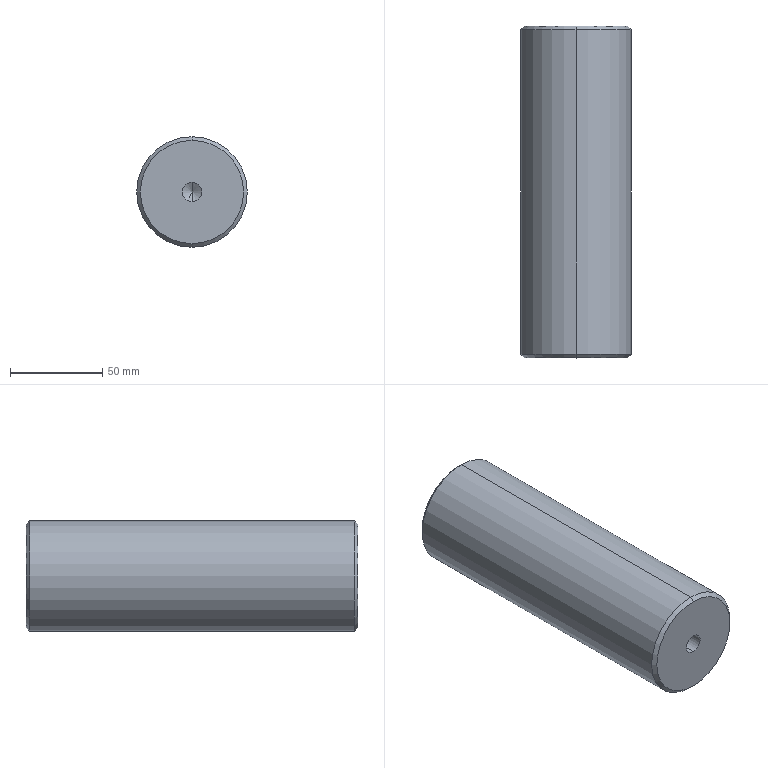Part | STEP file | Pilar - Torre - 1 cav. | 1 solid | 12 faces | box 60 x 180 x 60 mm | volume 505945 mm3 | cone 6 | cylinder 4 | plane 2 | commonest cylinder face diameters 10.5 x2 60 x2
STEP:
#1=CARTESIAN_POINT('',(0.,0.,0.));
#2=DIRECTION('',(0.,0.,1.));
#3=DIRECTION('',(1.,0.,0.));
#4=AXIS2_PLACEMENT_3D('',#1,#2,#3);
#5=CARTESIAN_POINT('',(0.,25.,-5.25));
#6=VERTEX_POINT('',#5);
#7=CARTESIAN_POINT('',(0.,0.,-5.25));
#8=VERTEX_POINT('',#7);
#9=CARTESIAN_POINT('',(0.,0.,-5.25));
#10=DIRECTION('',(0.,-1.,0.));
#11=VECTOR('',#10,1.);
#12=LINE('',#9,#11);
#13=CARTESIAN_POINT('',(0.,0.,0.));
#14=DIRECTION('',(0.,-1.,0.));
#15=DIRECTION('',(0.,0.,-1.));
#16=AXIS2_PLACEMENT_3D('',#13,#14,#15);
#17=CYLINDRICAL_SURFACE('',#16,5.25);
#18=CARTESIAN_POINT('',(6.283,0.));
#19=DIRECTION('',(0.,1.));
#20=VECTOR('',#19,1.);
#21=LINE('',#18,#20);
#22=(GEOMETRIC_REPRESENTATION_CONTEXT(2)PARAMETRIC_REPRESENTATION_CONTEXT()REPRESENTATION_CONTEXT('',''));
#23=DEFINITIONAL_REPRESENTATION('',(#21),#22);
#24=PCURVE('',#17,#23);
#25=CARTESIAN_POINT('',(0.,0.,0.));
#26=DIRECTION('',(0.,-1.,0.));
#27=DIRECTION('',(0.,0.,-1.));
#28=AXIS2_PLACEMENT_3D('',#25,#26,#27);
#29=CYLINDRICAL_SURFACE('',#28,5.25);
#30=CARTESIAN_POINT('',(0.,0.));
#31=DIRECTION('',(0.,1.));
#32=VECTOR('',#31,1.);
#33=LINE('',#30,#32);
#34=(GEOMETRIC_REPRESENTATION_CONTEXT(2)PARAMETRIC_REPRESENTATION_CONTEXT()REPRESENTATION_CONTEXT('',''));
#35=DEFINITIONAL_REPRESENTATION('',(#33),#34);
#36=PCURVE('',#29,#35);
#37=SURFACE_CURVE('',#12,(#24,#36),.PCURVE_S1.);
#38=EDGE_CURVE('',#6,#8,#37,.T.);
#39=ORIENTED_EDGE('',*,*,#38,.T.);
#40=CARTESIAN_POINT('',(0.,0.,5.25));
#41=VERTEX_POINT('',#40);
#42=CARTESIAN_POINT('',(0.,0.,0.));
#43=DIRECTION('',(0.,-1.,0.));
#44=DIRECTION('',(0.,0.,-1.));
#45=AXIS2_PLACEMENT_3D('',#42,#43,#44);
#46=CIRCLE('',#45,5.25);
#47=CARTESIAN_POINT('',(0.,0.));
#48=DIRECTION('',(1.,0.));
#49=VECTOR('',#48,1.);
#50=LINE('',#47,#49);
#51=(GEOMETRIC_REPRESENTATION_CONTEXT(2)PARAMETRIC_REPRESENTATION_CONTEXT()REPRESENTATION_CONTEXT('',''));
#52=DEFINITIONAL_REPRESENTATION('',(#50),#51);
#53=PCURVE('',#17,#52);
#54=CARTESIAN_POINT('',(0.,0.,0.));
#55=DIRECTION('',(0.,1.,0.));
#56=DIRECTION('',(0.,0.,1.));
#57=AXIS2_PLACEMENT_3D('',#54,#55,#56);
#58=PLANE('',#57);
#59=CARTESIAN_POINT('',(-5.25,0.));
#60=CARTESIAN_POINT('',(-5.25,9.093));
#61=CARTESIAN_POINT('',(2.625,4.547));
#62=CARTESIAN_POINT('',(10.5,0.));
#63=CARTESIAN_POINT('',(2.625,-4.547));
#64=CARTESIAN_POINT('',(-5.25,-9.093));
#65=CARTESIAN_POINT('',(-5.25,0.));
#66=(BOUNDED_CURVE()B_SPLINE_CURVE(2,(#59,#60,#61,#62,#63,#64,#65),.UNSPECIFIED.,.T.,.F.)B_SPLINE_CURVE_WITH_KNOTS((1,2,2,2,2,1),(-2.094,0.,2.094,4.189,6.283,8.378),.UNSPECIFIED.)CURVE()GEOMETRIC_REPRESENTATION_ITEM()RATIONAL_B_SPLINE_CURVE((1.,0.5,1.,0.5,1.,0.5,1.))REPRESENTATION_ITEM(''));
#67=(GEOMETRIC_REPRESENTATION_CONTEXT(2)PARAMETRIC_REPRESENTATION_CONTEXT()REPRESENTATION_CONTEXT('',''));
#68=DEFINITIONAL_REPRESENTATION('',(#66),#67);
#69=PCURVE('',#58,#68);
#70=SURFACE_CURVE('',#46,(#53,#69),.PCURVE_S1.);
#71=EDGE_CURVE('',#41,#8,#70,.T.);
#72=ORIENTED_EDGE('',*,*,#71,.F.);
#73=CARTESIAN_POINT('',(0.,25.,5.25));
#74=VERTEX_POINT('',#73);
#75=CARTESIAN_POINT('',(0.,0.,5.25));
#76=DIRECTION('',(0.,-1.,0.));
#77=VECTOR('',#76,1.);
#78=LINE('',#75,#77);
#79=CARTESIAN_POINT('',(3.142,0.));
#80=DIRECTION('',(0.,1.));
#81=VECTOR('',#80,1.);
#82=LINE('',#79,#81);
#83=(GEOMETRIC_REPRESENTATION_CONTEXT(2)PARAMETRIC_REPRESENTATION_CONTEXT()REPRESENTATION_CONTEXT('',''));
#84=DEFINITIONAL_REPRESENTATION('',(#82),#83);
#85=PCURVE('',#17,#84);
#86=CARTESIAN_POINT('',(3.142,0.));
#87=DIRECTION('',(0.,1.));
#88=VECTOR('',#87,1.);
#89=LINE('',#86,#88);
#90=(GEOMETRIC_REPRESENTATION_CONTEXT(2)PARAMETRIC_REPRESENTATION_CONTEXT()REPRESENTATION_CONTEXT('',''));
#91=DEFINITIONAL_REPRESENTATION('',(#89),#90);
#92=PCURVE('',#29,#91);
#93=SURFACE_CURVE('',#78,(#85,#92),.PCURVE_S1.);
#94=EDGE_CURVE('',#74,#41,#93,.T.);
#95=ORIENTED_EDGE('',*,*,#94,.F.);
#96=CARTESIAN_POINT('',(0.,25.,0.));
#97=DIRECTION('',(0.,-1.,0.));
#98=DIRECTION('',(0.,0.,-1.));
#99=AXIS2_PLACEMENT_3D('',#96,#97,#98);
#100=CIRCLE('',#99,5.25);
#101=CARTESIAN_POINT('',(0.,-25.));
#102=DIRECTION('',(1.,0.));
#103=VECTOR('',#102,1.);
#104=LINE('',#101,#103);
#105=(GEOMETRIC_REPRESENTATION_CONTEXT(2)PARAMETRIC_REPRESENTATION_CONTEXT()REPRESENTATION_CONTEXT('',''));
#106=DEFINITIONAL_REPRESENTATION('',(#104),#105);
#107=PCURVE('',#17,#106);
#108=CARTESIAN_POINT('',(0.,25.,0.));
#109=DIRECTION('',(0.,-1.,0.));
#110=DIRECTION('',(0.,0.,-1.));
#111=AXIS2_PLACEMENT_3D('',#108,#109,#110);
#112=CONICAL_SURFACE('',#111,5.25,1.03);
#113=CARTESIAN_POINT('',(0.,0.));
#114=DIRECTION('',(1.,0.));
#115=VECTOR('',#114,1.);
#116=LINE('',#113,#115);
#117=(GEOMETRIC_REPRESENTATION_CONTEXT(2)PARAMETRIC_REPRESENTATION_CONTEXT()REPRESENTATION_CONTEXT('',''));
#118=DEFINITIONAL_REPRESENTATION('',(#116),#117);
#119=PCURVE('',#112,#118);
#120=SURFACE_CURVE('',#100,(#107,#119),.PCURVE_S1.);
#121=EDGE_CURVE('',#74,#6,#120,.T.);
#122=ORIENTED_EDGE('',*,*,#121,.T.);
#123=EDGE_LOOP('',(#39,#72,#95,#122));
#124=FACE_BOUND('',#123,.F.);
#125=ADVANCED_FACE('',(#124),#17,.F.);
#126=ORIENTED_EDGE('',*,*,#121,.F.);
#127=CARTESIAN_POINT('',(0.,28.155,0.));
#128=VERTEX_POINT('',#127);
#129=CARTESIAN_POINT('',(0.,25.,5.25));
#130=DIRECTION('',(0.,-0.515,0.8572));
#131=VECTOR('',#130,1.);
#132=LINE('',#129,#131);
#133=CARTESIAN_POINT('',(3.142,0.));
#134=DIRECTION('',(0.,1.));
#135=VECTOR('',#134,1.);
#136=LINE('',#133,#135);
#137=(GEOMETRIC_REPRESENTATION_CONTEXT(2)PARAMETRIC_REPRESENTATION_CONTEXT()REPRESENTATION_CONTEXT('',''));
#138=DEFINITIONAL_REPRESENTATION('',(#136),#137);
#139=PCURVE('',#112,#138);
#140=CARTESIAN_POINT('',(0.,25.,0.));
#141=DIRECTION('',(0.,-1.,0.));
#142=DIRECTION('',(0.,0.,-1.));
#143=AXIS2_PLACEMENT_3D('',#140,#141,#142);
#144=CONICAL_SURFACE('',#143,5.25,1.03);
#145=CARTESIAN_POINT('',(3.142,0.));
#146=DIRECTION('',(0.,1.));
#147=VECTOR('',#146,1.);
#148=LINE('',#145,#147);
#149=(GEOMETRIC_REPRESENTATION_CONTEXT(2)PARAMETRIC_REPRESENTATION_CONTEXT()REPRESENTATION_CONTEXT('',''));
#150=DEFINITIONAL_REPRESENTATION('',(#148),#149);
#151=PCURVE('',#144,#150);
#152=SURFACE_CURVE('',#132,(#139,#151),.PCURVE_S1.);
#153=EDGE_CURVE('',#128,#74,#152,.T.);
#154=ORIENTED_EDGE('',*,*,#153,.F.);
#155=CARTESIAN_POINT('',(0.,25.,-5.25));
#156=DIRECTION('',(0.,-0.515,-0.8572));
#157=VECTOR('',#156,1.);
#158=LINE('',#155,#157);
#159=CARTESIAN_POINT('',(6.283,0.));
#160=DIRECTION('',(0.,1.));
#161=VECTOR('',#160,1.);
#162=LINE('',#159,#161);
#163=(GEOMETRIC_REPRESENTATION_CONTEXT(2)PARAMETRIC_REPRESENTATION_CONTEXT()REPRESENTATION_CONTEXT('',''));
#164=DEFINITIONAL_REPRESENTATION('',(#162),#163);
#165=PCURVE('',#112,#164);
#166=CARTESIAN_POINT('',(0.,0.));
#167=DIRECTION('',(0.,1.));
#168=VECTOR('',#167,1.);
#169=LINE('',#166,#168);
#170=(GEOMETRIC_REPRESENTATION_CONTEXT(2)PARAMETRIC_REPRESENTATION_CONTEXT()REPRESENTATION_CONTEXT('',''));
#171=DEFINITIONAL_REPRESENTATION('',(#169),#170);
#172=PCURVE('',#144,#171);
#173=SURFACE_CURVE('',#158,(#165,#172),.PCURVE_S1.);
#174=EDGE_CURVE('',#128,#6,#173,.T.);
#175=ORIENTED_EDGE('',*,*,#174,.T.);
#176=EDGE_LOOP('',(#126,#154,#175));
#177=FACE_BOUND('',#176,.F.);
#178=ADVANCED_FACE('',(#177),#112,.F.);
#179=CARTESIAN_POINT('',(0.,180.,28.));
#180=VERTEX_POINT('',#179);
#181=CARTESIAN_POINT('',(0.,180.,-28.));
#182=VERTEX_POINT('',#181);
#183=CARTESIAN_POINT('',(0.,180.,0.));
#184=DIRECTION('',(0.,1.,0.));
#185=DIRECTION('',(0.,0.,1.));
#186=AXIS2_PLACEMENT_3D('',#183,#184,#185);
#187=CIRCLE('',#186,28.);
#188=CARTESIAN_POINT('',(0.,180.,0.));
#189=DIRECTION('',(0.,-1.,0.));
#190=DIRECTION('',(0.,0.,-1.));
#191=AXIS2_PLACEMENT_3D('',#188,#189,#190);
#192=CONICAL_SURFACE('',#191,28.,0.7854);
#193=CARTESIAN_POINT('',(3.142,0.));
#194=DIRECTION('',(-1.,0.));
#195=VECTOR('',#194,1.);
#196=LINE('',#193,#195);
#197=(GEOMETRIC_REPRESENTATION_CONTEXT(2)PARAMETRIC_REPRESENTATION_CONTEXT()REPRESENTATION_CONTEXT('',''));
#198=DEFINITIONAL_REPRESENTATION('',(#196),#197);
#199=PCURVE('',#192,#198);
#200=CARTESIAN_POINT('',(0.,180.,0.));
#201=DIRECTION('',(0.,1.,0.));
#202=DIRECTION('',(0.,0.,1.));
#203=AXIS2_PLACEMENT_3D('',#200,#201,#202);
#204=PLANE('',#203);
#205=CARTESIAN_POINT('',(0.,0.));
#206=DIRECTION('',(1.,0.));
#207=AXIS2_PLACEMENT_2D('',#205,#206);
#208=CIRCLE('',#207,28.);
#209=(GEOMETRIC_REPRESENTATION_CONTEXT(2)PARAMETRIC_REPRESENTATION_CONTEXT()REPRESENTATION_CONTEXT('',''));
#210=DEFINITIONAL_REPRESENTATION('',(#208),#209);
#211=PCURVE('',#204,#210);
#212=SURFACE_CURVE('',#187,(#199,#211),.PCURVE_S1.);
#213=EDGE_CURVE('',#180,#182,#212,.T.);
#214=ORIENTED_EDGE('',*,*,#213,.F.);
#215=CARTESIAN_POINT('',(0.,178.,30.));
#216=VERTEX_POINT('',#215);
#217=CARTESIAN_POINT('',(0.,180.,28.));
#218=DIRECTION('',(0.,-0.7071,0.7071));
#219=VECTOR('',#218,1.);
#220=LINE('',#217,#219);
#221=CARTESIAN_POINT('',(3.142,0.));
#222=DIRECTION('',(0.,1.));
#223=VECTOR('',#222,1.);
#224=LINE('',#221,#223);
#225=(GEOMETRIC_REPRESENTATION_CONTEXT(2)PARAMETRIC_REPRESENTATION_CONTEXT()REPRESENTATION_CONTEXT('',''));
#226=DEFINITIONAL_REPRESENTATION('',(#224),#225);
#227=PCURVE('',#192,#226);
#228=CARTESIAN_POINT('',(0.,180.,0.));
#229=DIRECTION('',(0.,-1.,0.));
#230=DIRECTION('',(0.,0.,-1.));
#231=AXIS2_PLACEMENT_3D('',#228,#229,#230);
#232=CONICAL_SURFACE('',#231,28.,0.7854);
#233=CARTESIAN_POINT('',(3.142,0.));
#234=DIRECTION('',(0.,1.));
#235=VECTOR('',#234,1.);
#236=LINE('',#233,#235);
#237=(GEOMETRIC_REPRESENTATION_CONTEXT(2)PARAMETRIC_REPRESENTATION_CONTEXT()REPRESENTATION_CONTEXT('',''));
#238=DEFINITIONAL_REPRESENTATION('',(#236),#237);
#239=PCURVE('',#232,#238);
#240=SURFACE_CURVE('',#220,(#227,#239),.PCURVE_S1.);
#241=EDGE_CURVE('',#180,#216,#240,.T.);
#242=ORIENTED_EDGE('',*,*,#241,.T.);
#243=CARTESIAN_POINT('',(0.,178.,-30.));
#244=VERTEX_POINT('',#243);
#245=CARTESIAN_POINT('',(0.,178.,0.));
#246=DIRECTION('',(0.,-1.,0.));
#247=DIRECTION('',(0.,0.,1.));
#248=AXIS2_PLACEMENT_3D('',#245,#246,#247);
#249=CIRCLE('',#248,30.);
#250=CARTESIAN_POINT('',(-3.142,2.));
#251=DIRECTION('',(1.,0.));
#252=VECTOR('',#251,1.);
#253=LINE('',#250,#252);
#254=(GEOMETRIC_REPRESENTATION_CONTEXT(2)PARAMETRIC_REPRESENTATION_CONTEXT()REPRESENTATION_CONTEXT('',''));
#255=DEFINITIONAL_REPRESENTATION('',(#253),#254);
#256=PCURVE('',#192,#255);
#257=CARTESIAN_POINT('',(0.,180.,0.));
#258=DIRECTION('',(0.,-1.,0.));
#259=DIRECTION('',(0.,0.,-1.));
#260=AXIS2_PLACEMENT_3D('',#257,#258,#259);
#261=CYLINDRICAL_SURFACE('',#260,30.);
#262=CARTESIAN_POINT('',(-3.142,2.));
#263=DIRECTION('',(1.,0.));
#264=VECTOR('',#263,1.);
#265=LINE('',#262,#264);
#266=(GEOMETRIC_REPRESENTATION_CONTEXT(2)PARAMETRIC_REPRESENTATION_CONTEXT()REPRESENTATION_CONTEXT('',''));
#267=DEFINITIONAL_REPRESENTATION('',(#265),#266);
#268=PCURVE('',#261,#267);
#269=SURFACE_CURVE('',#249,(#256,#268),.PCURVE_S1.);
#270=EDGE_CURVE('',#244,#216,#269,.T.);
#271=ORIENTED_EDGE('',*,*,#270,.F.);
#272=CARTESIAN_POINT('',(0.,180.,-28.));
#273=DIRECTION('',(0.,-0.7071,-0.7071));
#274=VECTOR('',#273,1.);
#275=LINE('',#272,#274);
#276=CARTESIAN_POINT('',(0.,0.));
#277=DIRECTION('',(0.,1.));
#278=VECTOR('',#277,1.);
#279=LINE('',#276,#278);
#280=(GEOMETRIC_REPRESENTATION_CONTEXT(2)PARAMETRIC_REPRESENTATION_CONTEXT()REPRESENTATION_CONTEXT('',''));
#281=DEFINITIONAL_REPRESENTATION('',(#279),#280);
#282=PCURVE('',#192,#281);
#283=CARTESIAN_POINT('',(6.283,0.));
#284=DIRECTION('',(0.,1.));
#285=VECTOR('',#284,1.);
#286=LINE('',#283,#285);
#287=(GEOMETRIC_REPRESENTATION_CONTEXT(2)PARAMETRIC_REPRESENTATION_CONTEXT()REPRESENTATION_CONTEXT('',''));
#288=DEFINITIONAL_REPRESENTATION('',(#286),#287);
#289=PCURVE('',#232,#288);
#290=SURFACE_CURVE('',#275,(#282,#289),.PCURVE_S1.);
#291=EDGE_CURVE('',#182,#244,#290,.T.);
#292=ORIENTED_EDGE('',*,*,#291,.F.);
#293=EDGE_LOOP('',(#214,#242,#271,#292));
#294=FACE_BOUND('',#293,.T.);
#295=ADVANCED_FACE('',(#294),#192,.T.);
#296=CARTESIAN_POINT('',(0.,0.,-28.));
#297=VERTEX_POINT('',#296);
#298=CARTESIAN_POINT('',(0.,0.,28.));
#299=VERTEX_POINT('',#298);
#300=CARTESIAN_POINT('',(0.,0.,0.));
#301=DIRECTION('',(0.,-1.,0.));
#302=DIRECTION('',(0.,0.,1.));
#303=AXIS2_PLACEMENT_3D('',#300,#301,#302);
#304=CIRCLE('',#303,28.);
#305=CARTESIAN_POINT('',(0.,2.,0.));
#306=DIRECTION('',(0.,1.,0.));
#307=DIRECTION('',(0.,0.,1.));
#308=AXIS2_PLACEMENT_3D('',#305,#306,#307);
#309=CONICAL_SURFACE('',#308,30.,0.7854);
#310=CARTESIAN_POINT('',(6.283,-2.));
#311=DIRECTION('',(-1.,0.));
#312=VECTOR('',#311,1.);
#313=LINE('',#310,#312);
#314=(GEOMETRIC_REPRESENTATION_CONTEXT(2)PARAMETRIC_REPRESENTATION_CONTEXT()REPRESENTATION_CONTEXT('',''));
#315=DEFINITIONAL_REPRESENTATION('',(#313),#314);
#316=PCURVE('',#309,#315);
#317=CARTESIAN_POINT('',(28.,0.));
#318=CARTESIAN_POINT('',(28.,-48.497));
#319=CARTESIAN_POINT('',(-14.,-24.249));
#320=CARTESIAN_POINT('',(-56.,0.));
#321=CARTESIAN_POINT('',(-14.,24.249));
#322=CARTESIAN_POINT('',(28.,48.497));
#323=CARTESIAN_POINT('',(28.,0.));
#324=(BOUNDED_CURVE()B_SPLINE_CURVE(2,(#317,#318,#319,#320,#321,#322,#323),.UNSPECIFIED.,.T.,.F.)B_SPLINE_CURVE_WITH_KNOTS((1,2,2,2,2,1),(-2.094,0.,2.094,4.189,6.283,8.378),.UNSPECIFIED.)CURVE()GEOMETRIC_REPRESENTATION_ITEM()RATIONAL_B_SPLINE_CURVE((1.,0.5,1.,0.5,1.,0.5,1.))REPRESENTATION_ITEM(''));
#325=(GEOMETRIC_REPRESENTATION_CONTEXT(2)PARAMETRIC_REPRESENTATION_CONTEXT()REPRESENTATION_CONTEXT('',''));
#326=DEFINITIONAL_REPRESENTATION('',(#324),#325);
#327=PCURVE('',#58,#326);
#328=SURFACE_CURVE('',#304,(#316,#327),.PCURVE_S1.);
#329=EDGE_CURVE('',#297,#299,#328,.T.);
#330=ORIENTED_EDGE('',*,*,#329,.F.);
#331=CARTESIAN_POINT('',(0.,2.,-30.));
#332=VERTEX_POINT('',#331);
#333=CARTESIAN_POINT('',(0.,2.,-30.));
#334=DIRECTION('',(0.,0.7071,-0.7071));
#335=VECTOR('',#334,1.);
#336=LINE('',#333,#335);
#337=CARTESIAN_POINT('',(3.142,0.));
#338=DIRECTION('',(0.,1.));
#339=VECTOR('',#338,1.);
#340=LINE('',#337,#339);
#341=(GEOMETRIC_REPRESENTATION_CONTEXT(2)PARAMETRIC_REPRESENTATION_CONTEXT()REPRESENTATION_CONTEXT('',''));
#342=DEFINITIONAL_REPRESENTATION('',(#340),#341);
#343=PCURVE('',#309,#342);
#344=CARTESIAN_POINT('',(0.,2.,0.));
#345=DIRECTION('',(0.,1.,0.));
#346=DIRECTION('',(0.,0.,1.));
#347=AXIS2_PLACEMENT_3D('',#344,#345,#346);
#348=CONICAL_SURFACE('',#347,30.,0.7854);
#349=CARTESIAN_POINT('',(3.142,0.));
#350=DIRECTION('',(0.,1.));
#351=VECTOR('',#350,1.);
#352=LINE('',#349,#351);
#353=(GEOMETRIC_REPRESENTATION_CONTEXT(2)PARAMETRIC_REPRESENTATION_CONTEXT()REPRESENTATION_CONTEXT('',''));
#354=DEFINITIONAL_REPRESENTATION('',(#352),#353);
#355=PCURVE('',#348,#354);
#356=SURFACE_CURVE('',#336,(#343,#355),.PCURVE_S1.);
#357=EDGE_CURVE('',#297,#332,#356,.T.);
#358=ORIENTED_EDGE('',*,*,#357,.T.);
#359=CARTESIAN_POINT('',(0.,2.,30.));
#360=VERTEX_POINT('',#359);
#361=CARTESIAN_POINT('',(0.,2.,0.));
#362=DIRECTION('',(0.,1.,0.));
#363=DIRECTION('',(0.,0.,1.));
#364=AXIS2_PLACEMENT_3D('',#361,#362,#363);
#365=CIRCLE('',#364,30.);
#366=CARTESIAN_POINT('',(0.,0.));
#367=DIRECTION('',(1.,0.));
#368=VECTOR('',#367,1.);
#369=LINE('',#366,#368);
#370=(GEOMETRIC_REPRESENTATION_CONTEXT(2)PARAMETRIC_REPRESENTATION_CONTEXT()REPRESENTATION_CONTEXT('',''));
#371=DEFINITIONAL_REPRESENTATION('',(#369),#370);
#372=PCURVE('',#309,#371);
#373=CARTESIAN_POINT('',(3.142,178.));
#374=DIRECTION('',(-1.,0.));
#375=VECTOR('',#374,1.);
#376=LINE('',#373,#375);
#377=(GEOMETRIC_REPRESENTATION_CONTEXT(2)PARAMETRIC_REPRESENTATION_CONTEXT()REPRESENTATION_CONTEXT('',''));
#378=DEFINITIONAL_REPRESENTATION('',(#376),#377);
#379=PCURVE('',#261,#378);
#380=SURFACE_CURVE('',#365,(#372,#379),.PCURVE_S1.);
#381=EDGE_CURVE('',#360,#332,#380,.T.);
#382=ORIENTED_EDGE('',*,*,#381,.F.);
#383=CARTESIAN_POINT('',(0.,2.,30.));
#384=DIRECTION('',(0.,0.7071,0.7071));
#385=VECTOR('',#384,1.);
#386=LINE('',#383,#385);
#387=CARTESIAN_POINT('',(0.,0.));
#388=DIRECTION('',(0.,1.));
#389=VECTOR('',#388,1.);
#390=LINE('',#387,#389);
#391=(GEOMETRIC_REPRESENTATION_CONTEXT(2)PARAMETRIC_REPRESENTATION_CONTEXT()REPRESENTATION_CONTEXT('',''));
#392=DEFINITIONAL_REPRESENTATION('',(#390),#391);
#393=PCURVE('',#309,#392);
#394=CARTESIAN_POINT('',(6.283,0.));
#395=DIRECTION('',(0.,1.));
#396=VECTOR('',#395,1.);
#397=LINE('',#394,#396);
#398=(GEOMETRIC_REPRESENTATION_CONTEXT(2)PARAMETRIC_REPRESENTATION_CONTEXT()REPRESENTATION_CONTEXT('',''));
#399=DEFINITIONAL_REPRESENTATION('',(#397),#398);
#400=PCURVE('',#348,#399);
#401=SURFACE_CURVE('',#386,(#393,#400),.PCURVE_S1.);
#402=EDGE_CURVE('',#299,#360,#401,.T.);
#403=ORIENTED_EDGE('',*,*,#402,.F.);
#404=EDGE_LOOP('',(#330,#358,#382,#403));
#405=FACE_BOUND('',#404,.T.);
#406=ADVANCED_FACE('',(#405),#309,.T.);
#407=ORIENTED_EDGE('',*,*,#270,.T.);
#408=CARTESIAN_POINT('',(0.,180.,30.));
#409=DIRECTION('',(0.,-1.,0.));
#410=VECTOR('',#409,1.);
#411=LINE('',#408,#410);
#412=CARTESIAN_POINT('',(3.142,0.));
#413=DIRECTION('',(0.,1.));
#414=VECTOR('',#413,1.);
#415=LINE('',#412,#414);
#416=(GEOMETRIC_REPRESENTATION_CONTEXT(2)PARAMETRIC_REPRESENTATION_CONTEXT()REPRESENTATION_CONTEXT('',''));
#417=DEFINITIONAL_REPRESENTATION('',(#415),#416);
#418=PCURVE('',#261,#417);
#419=CARTESIAN_POINT('',(0.,180.,0.));
#420=DIRECTION('',(0.,-1.,0.));
#421=DIRECTION('',(0.,0.,-1.));
#422=AXIS2_PLACEMENT_3D('',#419,#420,#421);
#423=CYLINDRICAL_SURFACE('',#422,30.);
#424=CARTESIAN_POINT('',(3.142,0.));
#425=DIRECTION('',(0.,1.));
#426=VECTOR('',#425,1.);
#427=LINE('',#424,#426);
#428=(GEOMETRIC_REPRESENTATION_CONTEXT(2)PARAMETRIC_REPRESENTATION_CONTEXT()REPRESENTATION_CONTEXT('',''));
#429=DEFINITIONAL_REPRESENTATION('',(#427),#428);
#430=PCURVE('',#423,#429);
#431=SURFACE_CURVE('',#411,(#418,#430),.PCURVE_S1.);
#432=EDGE_CURVE('',#216,#360,#431,.T.);
#433=ORIENTED_EDGE('',*,*,#432,.T.);
#434=ORIENTED_EDGE('',*,*,#381,.T.);
#435=CARTESIAN_POINT('',(0.,180.,-30.));
#436=DIRECTION('',(0.,-1.,0.));
#437=VECTOR('',#436,1.);
#438=LINE('',#435,#437);
#439=CARTESIAN_POINT('',(0.,0.));
#440=DIRECTION('',(0.,1.));
#441=VECTOR('',#440,1.);
#442=LINE('',#439,#441);
#443=(GEOMETRIC_REPRESENTATION_CONTEXT(2)PARAMETRIC_REPRESENTATION_CONTEXT()REPRESENTATION_CONTEXT('',''));
#444=DEFINITIONAL_REPRESENTATION('',(#442),#443);
#445=PCURVE('',#261,#444);
#446=CARTESIAN_POINT('',(6.283,0.));
#447=DIRECTION('',(0.,1.));
#448=VECTOR('',#447,1.);
#449=LINE('',#446,#448);
#450=(GEOMETRIC_REPRESENTATION_CONTEXT(2)PARAMETRIC_REPRESENTATION_CONTEXT()REPRESENTATION_CONTEXT('',''));
#451=DEFINITIONAL_REPRESENTATION('',(#449),#450);
#452=PCURVE('',#423,#451);
#453=SURFACE_CURVE('',#438,(#445,#452),.PCURVE_S1.);
#454=EDGE_CURVE('',#244,#332,#453,.T.);
#455=ORIENTED_EDGE('',*,*,#454,.F.);
#456=EDGE_LOOP('',(#407,#433,#434,#455));
#457=FACE_BOUND('',#456,.T.);
#458=ADVANCED_FACE('',(#457),#261,.T.);
#459=ORIENTED_EDGE('',*,*,#432,.F.);
#460=CARTESIAN_POINT('',(0.,178.,0.));
#461=DIRECTION('',(0.,-1.,0.));
#462=DIRECTION('',(0.,0.,1.));
#463=AXIS2_PLACEMENT_3D('',#460,#461,#462);
#464=CIRCLE('',#463,30.);
#465=CARTESIAN_POINT('',(3.142,2.));
#466=DIRECTION('',(1.,0.));
#467=VECTOR('',#466,1.);
#468=LINE('',#465,#467);
#469=(GEOMETRIC_REPRESENTATION_CONTEXT(2)PARAMETRIC_REPRESENTATION_CONTEXT()REPRESENTATION_CONTEXT('',''));
#470=DEFINITIONAL_REPRESENTATION('',(#468),#469);
#471=PCURVE('',#423,#470);
#472=CARTESIAN_POINT('',(3.142,2.));
#473=DIRECTION('',(1.,0.));
#474=VECTOR('',#473,1.);
#475=LINE('',#472,#474);
#476=(GEOMETRIC_REPRESENTATION_CONTEXT(2)PARAMETRIC_REPRESENTATION_CONTEXT()REPRESENTATION_CONTEXT('',''));
#477=DEFINITIONAL_REPRESENTATION('',(#475),#476);
#478=PCURVE('',#232,#477);
#479=SURFACE_CURVE('',#464,(#471,#478),.PCURVE_S1.);
#480=EDGE_CURVE('',#216,#244,#479,.T.);
#481=ORIENTED_EDGE('',*,*,#480,.T.);
#482=ORIENTED_EDGE('',*,*,#454,.T.);
#483=CARTESIAN_POINT('',(0.,2.,0.));
#484=DIRECTION('',(0.,1.,0.));
#485=DIRECTION('',(0.,0.,1.));
#486=AXIS2_PLACEMENT_3D('',#483,#484,#485);
#487=CIRCLE('',#486,30.);
#488=CARTESIAN_POINT('',(9.425,178.));
#489=DIRECTION('',(-1.,0.));
#490=VECTOR('',#489,1.);
#491=LINE('',#488,#490);
#492=(GEOMETRIC_REPRESENTATION_CONTEXT(2)PARAMETRIC_REPRESENTATION_CONTEXT()REPRESENTATION_CONTEXT('',''));
#493=DEFINITIONAL_REPRESENTATION('',(#491),#492);
#494=PCURVE('',#423,#493);
#495=CARTESIAN_POINT('',(0.,0.));
#496=DIRECTION('',(1.,0.));
#497=VECTOR('',#496,1.);
#498=LINE('',#495,#497);
#499=(GEOMETRIC_REPRESENTATION_CONTEXT(2)PARAMETRIC_REPRESENTATION_CONTEXT()REPRESENTATION_CONTEXT('',''));
#500=DEFINITIONAL_REPRESENTATION('',(#498),#499);
#501=PCURVE('',#348,#500);
#502=SURFACE_CURVE('',#487,(#494,#501),.PCURVE_S1.);
#503=EDGE_CURVE('',#332,#360,#502,.T.);
#504=ORIENTED_EDGE('',*,*,#503,.T.);
#505=EDGE_LOOP('',(#459,#481,#482,#504));
#506=FACE_BOUND('',#505,.T.);
#507=ADVANCED_FACE('',(#506),#423,.T.);
#508=CARTESIAN_POINT('',(0.,180.,0.));
#509=DIRECTION('',(0.,1.,0.));
#510=DIRECTION('',(0.,0.,1.));
#511=AXIS2_PLACEMENT_3D('',#508,#509,#510);
#512=CIRCLE('',#511,28.);
#513=CARTESIAN_POINT('',(0.,0.));
#514=DIRECTION('',(1.,0.));
#515=AXIS2_PLACEMENT_2D('',#513,#514);
#516=CIRCLE('',#515,28.);
#517=(GEOMETRIC_REPRESENTATION_CONTEXT(2)PARAMETRIC_REPRESENTATION_CONTEXT()REPRESENTATION_CONTEXT('',''));
#518=DEFINITIONAL_REPRESENTATION('',(#516),#517);
#519=PCURVE('',#204,#518);
#520=CARTESIAN_POINT('',(9.425,0.));
#521=DIRECTION('',(-1.,0.));
#522=VECTOR('',#521,1.);
#523=LINE('',#520,#522);
#524=(GEOMETRIC_REPRESENTATION_CONTEXT(2)PARAMETRIC_REPRESENTATION_CONTEXT()REPRESENTATION_CONTEXT('',''));
#525=DEFINITIONAL_REPRESENTATION('',(#523),#524);
#526=PCURVE('',#232,#525);
#527=SURFACE_CURVE('',#512,(#519,#526),.PCURVE_S1.);
#528=EDGE_CURVE('',#182,#180,#527,.T.);
#529=ORIENTED_EDGE('',*,*,#528,.T.);
#530=ORIENTED_EDGE('',*,*,#213,.T.);
#531=EDGE_LOOP('',(#529,#530));
#532=FACE_BOUND('',#531,.T.);
#533=ADVANCED_FACE('',(#532),#204,.T.);
#534=CARTESIAN_POINT('',(0.,0.,0.));
#535=DIRECTION('',(0.,-1.,0.));
#536=DIRECTION('',(0.,0.,-1.));
#537=AXIS2_PLACEMENT_3D('',#534,#535,#536);
#538=CIRCLE('',#537,5.25);
#539=CARTESIAN_POINT('',(-5.25,0.));
#540=CARTESIAN_POINT('',(-5.25,9.093));
#541=CARTESIAN_POINT('',(2.625,4.547));
#542=CARTESIAN_POINT('',(10.5,0.));
#543=CARTESIAN_POINT('',(2.625,-4.547));
#544=CARTESIAN_POINT('',(-5.25,-9.093));
#545=CARTESIAN_POINT('',(-5.25,0.));
#546=(BOUNDED_CURVE()B_SPLINE_CURVE(2,(#539,#540,#541,#542,#543,#544,#545),.UNSPECIFIED.,.T.,.F.)B_SPLINE_CURVE_WITH_KNOTS((1,2,2,2,2,1),(-2.094,0.,2.094,4.189,6.283,8.378),.UNSPECIFIED.)CURVE()GEOMETRIC_REPRESENTATION_ITEM()RATIONAL_B_SPLINE_CURVE((1.,0.5,1.,0.5,1.,0.5,1.))REPRESENTATION_ITEM(''));
#547=(GEOMETRIC_REPRESENTATION_CONTEXT(2)PARAMETRIC_REPRESENTATION_CONTEXT()REPRESENTATION_CONTEXT('',''));
#548=DEFINITIONAL_REPRESENTATION('',(#546),#547);
#549=PCURVE('',#58,#548);
#550=CARTESIAN_POINT('',(0.,0.));
#551=DIRECTION('',(1.,0.));
#552=VECTOR('',#551,1.);
#553=LINE('',#550,#552);
#554=(GEOMETRIC_REPRESENTATION_CONTEXT(2)PARAMETRIC_REPRESENTATION_CONTEXT()REPRESENTATION_CONTEXT('',''));
#555=DEFINITIONAL_REPRESENTATION('',(#553),#554);
#556=PCURVE('',#29,#555);
#557=SURFACE_CURVE('',#538,(#549,#556),.PCURVE_S1.);
#558=EDGE_CURVE('',#8,#41,#557,.T.);
#559=ORIENTED_EDGE('',*,*,#558,.F.);
#560=ORIENTED_EDGE('',*,*,#71,.F.);
#561=EDGE_LOOP('',(#559,#560));
#562=FACE_BOUND('',#561,.T.);
#563=CARTESIAN_POINT('',(0.,0.,0.));
#564=DIRECTION('',(0.,-1.,0.));
#565=DIRECTION('',(0.,0.,1.));
#566=AXIS2_PLACEMENT_3D('',#563,#564,#565);
#567=CIRCLE('',#566,28.);
#568=CARTESIAN_POINT('',(28.,0.));
#569=CARTESIAN_POINT('',(28.,-48.497));
#570=CARTESIAN_POINT('',(-14.,-24.249));
#571=CARTESIAN_POINT('',(-56.,0.));
#572=CARTESIAN_POINT('',(-14.,24.249));
#573=CARTESIAN_POINT('',(28.,48.497));
#574=CARTESIAN_POINT('',(28.,0.));
#575=(BOUNDED_CURVE()B_SPLINE_CURVE(2,(#568,#569,#570,#571,#572,#573,#574),.UNSPECIFIED.,.T.,.F.)B_SPLINE_CURVE_WITH_KNOTS((1,2,2,2,2,1),(-2.094,0.,2.094,4.189,6.283,8.378),.UNSPECIFIED.)CURVE()GEOMETRIC_REPRESENTATION_ITEM()RATIONAL_B_SPLINE_CURVE((1.,0.5,1.,0.5,1.,0.5,1.))REPRESENTATION_ITEM(''));
#576=(GEOMETRIC_REPRESENTATION_CONTEXT(2)PARAMETRIC_REPRESENTATION_CONTEXT()REPRESENTATION_CONTEXT('',''));
#577=DEFINITIONAL_REPRESENTATION('',(#575),#576);
#578=PCURVE('',#58,#577);
#579=CARTESIAN_POINT('',(6.283,-2.));
#580=DIRECTION('',(-1.,0.));
#581=VECTOR('',#580,1.);
#582=LINE('',#579,#581);
#583=(GEOMETRIC_REPRESENTATION_CONTEXT(2)PARAMETRIC_REPRESENTATION_CONTEXT()REPRESENTATION_CONTEXT('',''));
#584=DEFINITIONAL_REPRESENTATION('',(#582),#583);
#585=PCURVE('',#348,#584);
#586=SURFACE_CURVE('',#567,(#578,#585),.PCURVE_S1.);
#587=EDGE_CURVE('',#299,#297,#586,.T.);
#588=ORIENTED_EDGE('',*,*,#587,.T.);
#589=ORIENTED_EDGE('',*,*,#329,.T.);
#590=EDGE_LOOP('',(#588,#589));
#591=FACE_BOUND('',#590,.T.);
#592=ADVANCED_FACE('',(#562,#591),#58,.F.);
#593=ORIENTED_EDGE('',*,*,#357,.F.);
#594=ORIENTED_EDGE('',*,*,#587,.F.);
#595=ORIENTED_EDGE('',*,*,#402,.T.);
#596=ORIENTED_EDGE('',*,*,#503,.F.);
#597=EDGE_LOOP('',(#593,#594,#595,#596));
#598=FACE_BOUND('',#597,.T.);
#599=ADVANCED_FACE('',(#598),#348,.T.);
#600=ORIENTED_EDGE('',*,*,#241,.F.);
#601=ORIENTED_EDGE('',*,*,#528,.F.);
#602=ORIENTED_EDGE('',*,*,#291,.T.);
#603=ORIENTED_EDGE('',*,*,#480,.F.);
#604=EDGE_LOOP('',(#600,#601,#602,#603));
#605=FACE_BOUND('',#604,.T.);
#606=ADVANCED_FACE('',(#605),#232,.T.);
#607=CARTESIAN_POINT('',(0.,25.,0.));
#608=DIRECTION('',(0.,-1.,0.));
#609=DIRECTION('',(0.,0.,-1.));
#610=AXIS2_PLACEMENT_3D('',#607,#608,#609);
#611=CIRCLE('',#610,5.25);
#612=CARTESIAN_POINT('',(0.,0.));
#613=DIRECTION('',(1.,0.));
#614=VECTOR('',#613,1.);
#615=LINE('',#612,#614);
#616=(GEOMETRIC_REPRESENTATION_CONTEXT(2)PARAMETRIC_REPRESENTATION_CONTEXT()REPRESENTATION_CONTEXT('',''));
#617=DEFINITIONAL_REPRESENTATION('',(#615),#616);
#618=PCURVE('',#144,#617);
#619=CARTESIAN_POINT('',(0.,-25.));
#620=DIRECTION('',(1.,0.));
#621=VECTOR('',#620,1.);
#622=LINE('',#619,#621);
#623=(GEOMETRIC_REPRESENTATION_CONTEXT(2)PARAMETRIC_REPRESENTATION_CONTEXT()REPRESENTATION_CONTEXT('',''));
#624=DEFINITIONAL_REPRESENTATION('',(#622),#623);
#625=PCURVE('',#29,#624);
#626=SURFACE_CURVE('',#611,(#618,#625),.PCURVE_S1.);
#627=EDGE_CURVE('',#6,#74,#626,.T.);
#628=ORIENTED_EDGE('',*,*,#627,.F.);
#629=ORIENTED_EDGE('',*,*,#174,.F.);
#630=ORIENTED_EDGE('',*,*,#153,.T.);
#631=EDGE_LOOP('',(#628,#629,#630));
#632=FACE_BOUND('',#631,.F.);
#633=ADVANCED_FACE('',(#632),#144,.F.);
#634=ORIENTED_EDGE('',*,*,#558,.F.);
#635=ORIENTED_EDGE('',*,*,#38,.F.);
#636=ORIENTED_EDGE('',*,*,#627,.T.);
#637=ORIENTED_EDGE('',*,*,#94,.T.);
#638=EDGE_LOOP('',(#634,#635,#636,#637));
#639=FACE_BOUND('',#638,.F.);
#640=ADVANCED_FACE('',(#639),#29,.F.);
#641=CLOSED_SHELL('',(#125,#178,#295,#406,#458,#507,#533,#592,#599,#606,#633,#640));
#642=MANIFOLD_SOLID_BREP('',#641);
#643=(LENGTH_UNIT()NAMED_UNIT(*)SI_UNIT(.MILLI.,.METRE.));
#644=UNCERTAINTY_MEASURE_WITH_UNIT(LENGTH_MEASURE(0.0000001),#643,'','');
#645=(NAMED_UNIT(*)PLANE_ANGLE_UNIT()SI_UNIT($,.RADIAN.));
#646=(NAMED_UNIT(*)SI_UNIT($,.STERADIAN.)SOLID_ANGLE_UNIT());
#647=(GEOMETRIC_REPRESENTATION_CONTEXT(3)GLOBAL_UNCERTAINTY_ASSIGNED_CONTEXT((#644))GLOBAL_UNIT_ASSIGNED_CONTEXT((#643,#645,#646))REPRESENTATION_CONTEXT('',''));
#648=ADVANCED_BREP_SHAPE_REPRESENTATION('',(#4,#642),#647);